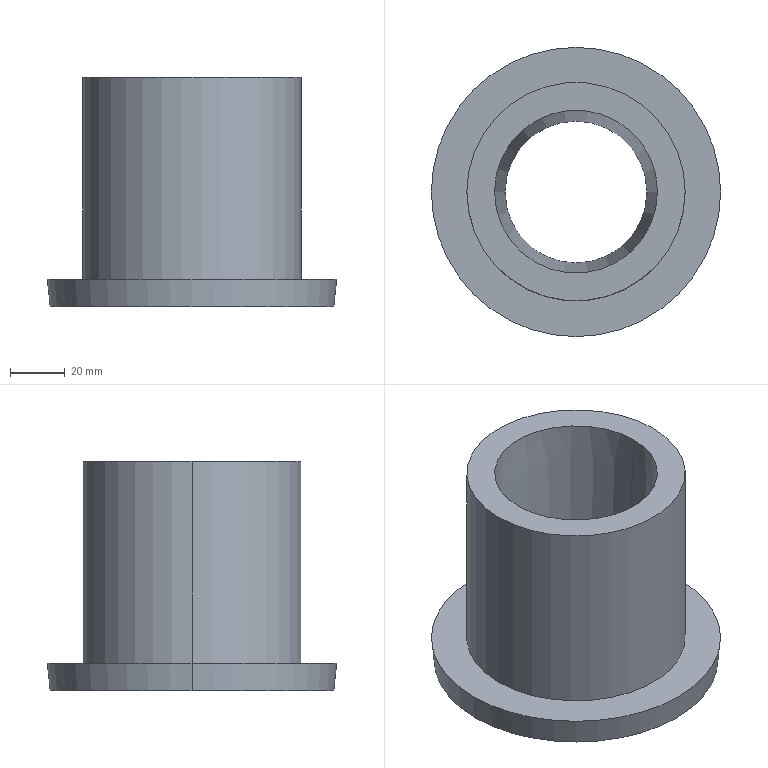Part | SolidWorks | features Revolution 1 | 1 solid | 9 faces | box 106 x 106 x 84 mm | volume 252355 mm3 | cone 4 | plane 3 | cylinder 2 | commonest cylinder face diameters 80 x2
STEP:
#1=CARTESIAN_POINT('',(-40.,318.5,-90.5));
#2=VERTEX_POINT('',#1);
#3=CARTESIAN_POINT('',(40.,318.5,-90.5));
#4=VERTEX_POINT('',#3);
#5=CARTESIAN_POINT('',(0.,318.5,-90.5));
#6=DIRECTION('',(0.,0.,-1.));
#7=DIRECTION('',(-1.,0.,0.));
#8=AXIS2_PLACEMENT_3D('',#5,#6,#7);
#9=CIRCLE('',#8,40.);
#10=EDGE_CURVE('',#2,#4,#9,.T.);
#11=ORIENTED_EDGE('',*,*,#10,.T.);
#12=CARTESIAN_POINT('',(40.,318.5,-164.5));
#13=VERTEX_POINT('',#12);
#14=CARTESIAN_POINT('',(40.,318.5,-174.5));
#15=DIRECTION('',(0.,0.,-1.));
#16=VECTOR('',#15,1000.);
#17=LINE('',#14,#16);
#18=EDGE_CURVE('',#4,#13,#17,.T.);
#19=ORIENTED_EDGE('',*,*,#18,.T.);
#20=CARTESIAN_POINT('',(-40.,318.5,-164.5));
#21=VERTEX_POINT('',#20);
#22=CARTESIAN_POINT('',(0.,318.5,-164.5));
#23=DIRECTION('',(0.,0.,-1.));
#24=DIRECTION('',(-1.,0.,0.));
#25=AXIS2_PLACEMENT_3D('',#22,#23,#24);
#26=CIRCLE('',#25,40.);
#27=EDGE_CURVE('',#21,#13,#26,.T.);
#28=ORIENTED_EDGE('',*,*,#27,.F.);
#29=CARTESIAN_POINT('',(-40.,318.5,-174.5));
#30=DIRECTION('',(0.,0.,-1.));
#31=VECTOR('',#30,1000.);
#32=LINE('',#29,#31);
#33=EDGE_CURVE('',#2,#21,#32,.T.);
#34=ORIENTED_EDGE('',*,*,#33,.F.);
#35=EDGE_LOOP('',(#11,#19,#28,#34));
#36=FACE_OUTER_BOUND('',#35,.T.);
#37=CARTESIAN_POINT('',(0.,318.5,-174.5));
#38=DIRECTION('',(0.,0.,-1.));
#39=DIRECTION('',(-1.,0.,0.));
#40=AXIS2_PLACEMENT_3D('',#37,#38,#39);
#41=CYLINDRICAL_SURFACE('',#40,40.);
#42=ADVANCED_FACE('',(#36),#41,.T.);
#43=CARTESIAN_POINT('',(-52.,318.5,-174.5));
#44=VERTEX_POINT('',#43);
#45=CARTESIAN_POINT('',(52.,318.5,-174.5));
#46=VERTEX_POINT('',#45);
#47=CARTESIAN_POINT('',(0.,318.5,-174.5));
#48=DIRECTION('',(0.,0.,-1.));
#49=DIRECTION('',(-1.,0.,0.));
#50=AXIS2_PLACEMENT_3D('',#47,#48,#49);
#51=CIRCLE('',#50,52.);
#52=EDGE_CURVE('',#44,#46,#51,.T.);
#53=ORIENTED_EDGE('',*,*,#52,.F.);
#54=CARTESIAN_POINT('',(-53.,318.5,-164.5));
#55=VERTEX_POINT('',#54);
#56=CARTESIAN_POINT('',(-53.,318.5,-164.5));
#57=DIRECTION('',(-0.0995,0.,0.995));
#58=VECTOR('',#57,1000.);
#59=LINE('',#56,#58);
#60=EDGE_CURVE('',#44,#55,#59,.T.);
#61=ORIENTED_EDGE('',*,*,#60,.T.);
#62=CARTESIAN_POINT('',(53.,318.5,-164.5));
#63=VERTEX_POINT('',#62);
#64=CARTESIAN_POINT('',(0.,318.5,-164.5));
#65=DIRECTION('',(0.,0.,-1.));
#66=DIRECTION('',(-1.,0.,0.));
#67=AXIS2_PLACEMENT_3D('',#64,#65,#66);
#68=CIRCLE('',#67,53.);
#69=EDGE_CURVE('',#55,#63,#68,.T.);
#70=ORIENTED_EDGE('',*,*,#69,.T.);
#71=CARTESIAN_POINT('',(53.,318.5,-164.5));
#72=DIRECTION('',(0.0995,0.,0.995));
#73=VECTOR('',#72,1000.);
#74=LINE('',#71,#73);
#75=EDGE_CURVE('',#46,#63,#74,.T.);
#76=ORIENTED_EDGE('',*,*,#75,.F.);
#77=EDGE_LOOP('',(#53,#61,#70,#76));
#78=FACE_OUTER_BOUND('',#77,.T.);
#79=CARTESIAN_POINT('',(0.,318.5,-164.5));
#80=DIRECTION('',(0.,0.,1.));
#81=DIRECTION('',(1.,0.,0.));
#82=AXIS2_PLACEMENT_3D('',#79,#80,#81);
#83=CONICAL_SURFACE('',#82,53.,0.09967);
#84=ADVANCED_FACE('',(#78),#83,.T.);
#85=CARTESIAN_POINT('',(26.,318.5,-174.5));
#86=VERTEX_POINT('',#85);
#87=CARTESIAN_POINT('',(-26.,318.5,-174.5));
#88=VERTEX_POINT('',#87);
#89=CARTESIAN_POINT('',(0.,318.5,-174.5));
#90=DIRECTION('',(0.,0.,-1.));
#91=DIRECTION('',(-1.,0.,0.));
#92=AXIS2_PLACEMENT_3D('',#89,#90,#91);
#93=CIRCLE('',#92,26.);
#94=EDGE_CURVE('',#86,#88,#93,.T.);
#95=ORIENTED_EDGE('',*,*,#94,.T.);
#96=CARTESIAN_POINT('',(-29.862,318.5,-90.5));
#97=VERTEX_POINT('',#96);
#98=CARTESIAN_POINT('',(-26.,318.5,-174.5));
#99=DIRECTION('',(-0.04593,0.,0.9989));
#100=VECTOR('',#99,1000.);
#101=LINE('',#98,#100);
#102=EDGE_CURVE('',#88,#97,#101,.T.);
#103=ORIENTED_EDGE('',*,*,#102,.T.);
#104=CARTESIAN_POINT('',(29.862,318.5,-90.5));
#105=VERTEX_POINT('',#104);
#106=CARTESIAN_POINT('',(0.,318.5,-90.5));
#107=DIRECTION('',(0.,0.,-1.));
#108=DIRECTION('',(-1.,0.,0.));
#109=AXIS2_PLACEMENT_3D('',#106,#107,#108);
#110=CIRCLE('',#109,29.862);
#111=EDGE_CURVE('',#105,#97,#110,.T.);
#112=ORIENTED_EDGE('',*,*,#111,.F.);
#113=CARTESIAN_POINT('',(26.,318.5,-174.5));
#114=DIRECTION('',(0.04593,0.,0.9989));
#115=VECTOR('',#114,1000.);
#116=LINE('',#113,#115);
#117=EDGE_CURVE('',#86,#105,#116,.T.);
#118=ORIENTED_EDGE('',*,*,#117,.F.);
#119=EDGE_LOOP('',(#95,#103,#112,#118));
#120=FACE_OUTER_BOUND('',#119,.T.);
#121=CARTESIAN_POINT('',(0.,318.5,-174.5));
#122=DIRECTION('',(0.,0.,1.));
#123=DIRECTION('',(1.,0.,0.));
#124=AXIS2_PLACEMENT_3D('',#121,#122,#123);
#125=CONICAL_SURFACE('',#124,26.,0.04594);
#126=ADVANCED_FACE('',(#120),#125,.F.);
#127=ORIENTED_EDGE('',*,*,#102,.F.);
#128=CARTESIAN_POINT('',(0.,318.5,-174.5));
#129=DIRECTION('',(0.,0.,-1.));
#130=DIRECTION('',(-1.,0.,0.));
#131=AXIS2_PLACEMENT_3D('',#128,#129,#130);
#132=CIRCLE('',#131,26.);
#133=EDGE_CURVE('',#88,#86,#132,.T.);
#134=ORIENTED_EDGE('',*,*,#133,.T.);
#135=ORIENTED_EDGE('',*,*,#117,.T.);
#136=CARTESIAN_POINT('',(0.,318.5,-90.5));
#137=DIRECTION('',(0.,0.,-1.));
#138=DIRECTION('',(-1.,0.,0.));
#139=AXIS2_PLACEMENT_3D('',#136,#137,#138);
#140=CIRCLE('',#139,29.862);
#141=EDGE_CURVE('',#97,#105,#140,.T.);
#142=ORIENTED_EDGE('',*,*,#141,.F.);
#143=EDGE_LOOP('',(#127,#134,#135,#142));
#144=FACE_OUTER_BOUND('',#143,.T.);
#145=CARTESIAN_POINT('',(0.,318.5,-174.5));
#146=DIRECTION('',(0.,0.,1.));
#147=DIRECTION('',(1.,0.,0.));
#148=AXIS2_PLACEMENT_3D('',#145,#146,#147);
#149=CONICAL_SURFACE('',#148,26.,0.04594);
#150=ADVANCED_FACE('',(#144),#149,.F.);
#151=ORIENTED_EDGE('',*,*,#94,.F.);
#152=ORIENTED_EDGE('',*,*,#133,.F.);
#153=EDGE_LOOP('',(#151,#152));
#154=FACE_BOUND('',#153,.T.);
#155=CARTESIAN_POINT('',(0.,318.5,-174.5));
#156=DIRECTION('',(0.,0.,-1.));
#157=DIRECTION('',(-1.,0.,0.));
#158=AXIS2_PLACEMENT_3D('',#155,#156,#157);
#159=CIRCLE('',#158,52.);
#160=EDGE_CURVE('',#46,#44,#159,.T.);
#161=ORIENTED_EDGE('',*,*,#160,.T.);
#162=ORIENTED_EDGE('',*,*,#52,.T.);
#163=EDGE_LOOP('',(#161,#162));
#164=FACE_OUTER_BOUND('',#163,.T.);
#165=CARTESIAN_POINT('',(-26.,318.5,-174.5));
#166=DIRECTION('',(0.,0.,1.));
#167=DIRECTION('',(1.,0.,0.));
#168=AXIS2_PLACEMENT_3D('',#165,#166,#167);
#169=PLANE('',#168);
#170=ADVANCED_FACE('',(#154,#164),#169,.F.);
#171=ORIENTED_EDGE('',*,*,#60,.F.);
#172=ORIENTED_EDGE('',*,*,#160,.F.);
#173=ORIENTED_EDGE('',*,*,#75,.T.);
#174=CARTESIAN_POINT('',(0.,318.5,-164.5));
#175=DIRECTION('',(0.,0.,-1.));
#176=DIRECTION('',(-1.,0.,0.));
#177=AXIS2_PLACEMENT_3D('',#174,#175,#176);
#178=CIRCLE('',#177,53.);
#179=EDGE_CURVE('',#63,#55,#178,.T.);
#180=ORIENTED_EDGE('',*,*,#179,.T.);
#181=EDGE_LOOP('',(#171,#172,#173,#180));
#182=FACE_OUTER_BOUND('',#181,.T.);
#183=CARTESIAN_POINT('',(0.,318.5,-164.5));
#184=DIRECTION('',(0.,0.,1.));
#185=DIRECTION('',(1.,0.,0.));
#186=AXIS2_PLACEMENT_3D('',#183,#184,#185);
#187=CONICAL_SURFACE('',#186,53.,0.09967);
#188=ADVANCED_FACE('',(#182),#187,.T.);
#189=ORIENTED_EDGE('',*,*,#179,.F.);
#190=ORIENTED_EDGE('',*,*,#69,.F.);
#191=EDGE_LOOP('',(#189,#190));
#192=FACE_OUTER_BOUND('',#191,.T.);
#193=ORIENTED_EDGE('',*,*,#27,.T.);
#194=CARTESIAN_POINT('',(0.,318.5,-164.5));
#195=DIRECTION('',(0.,0.,-1.));
#196=DIRECTION('',(-1.,0.,0.));
#197=AXIS2_PLACEMENT_3D('',#194,#195,#196);
#198=CIRCLE('',#197,40.);
#199=EDGE_CURVE('',#13,#21,#198,.T.);
#200=ORIENTED_EDGE('',*,*,#199,.T.);
#201=EDGE_LOOP('',(#193,#200));
#202=FACE_BOUND('',#201,.T.);
#203=CARTESIAN_POINT('',(-53.,318.5,-164.5));
#204=DIRECTION('',(0.,0.,-1.));
#205=DIRECTION('',(-1.,0.,0.));
#206=AXIS2_PLACEMENT_3D('',#203,#204,#205);
#207=PLANE('',#206);
#208=ADVANCED_FACE('',(#192,#202),#207,.F.);
#209=ORIENTED_EDGE('',*,*,#18,.F.);
#210=CARTESIAN_POINT('',(0.,318.5,-90.5));
#211=DIRECTION('',(0.,0.,-1.));
#212=DIRECTION('',(-1.,0.,0.));
#213=AXIS2_PLACEMENT_3D('',#210,#211,#212);
#214=CIRCLE('',#213,40.);
#215=EDGE_CURVE('',#4,#2,#214,.T.);
#216=ORIENTED_EDGE('',*,*,#215,.T.);
#217=ORIENTED_EDGE('',*,*,#33,.T.);
#218=ORIENTED_EDGE('',*,*,#199,.F.);
#219=EDGE_LOOP('',(#209,#216,#217,#218));
#220=FACE_OUTER_BOUND('',#219,.T.);
#221=CARTESIAN_POINT('',(0.,318.5,-174.5));
#222=DIRECTION('',(0.,0.,-1.));
#223=DIRECTION('',(-1.,0.,0.));
#224=AXIS2_PLACEMENT_3D('',#221,#222,#223);
#225=CYLINDRICAL_SURFACE('',#224,40.);
#226=ADVANCED_FACE('',(#220),#225,.T.);
#227=ORIENTED_EDGE('',*,*,#10,.F.);
#228=ORIENTED_EDGE('',*,*,#215,.F.);
#229=EDGE_LOOP('',(#227,#228));
#230=FACE_OUTER_BOUND('',#229,.T.);
#231=ORIENTED_EDGE('',*,*,#111,.T.);
#232=ORIENTED_EDGE('',*,*,#141,.T.);
#233=EDGE_LOOP('',(#231,#232));
#234=FACE_BOUND('',#233,.T.);
#235=CARTESIAN_POINT('',(-40.,318.5,-90.5));
#236=DIRECTION('',(0.,0.,-1.));
#237=DIRECTION('',(-1.,0.,0.));
#238=AXIS2_PLACEMENT_3D('',#235,#236,#237);
#239=PLANE('',#238);
#240=ADVANCED_FACE('',(#230,#234),#239,.F.);
#241=CLOSED_SHELL('',(#42,#84,#126,#150,#170,#188,#208,#226,#240));
#242=MANIFOLD_SOLID_BREP('',#241);
#243=CARTESIAN_POINT('',(0.,0.,0.));
#244=DIRECTION('',(0.,0.,1.));
#245=DIRECTION('',(1.,0.,0.));
#246=AXIS2_PLACEMENT_3D('',#243,#244,#245);
#247=(LENGTH_UNIT()NAMED_UNIT(*)SI_UNIT(.MILLI.,.METRE.));
#248=UNCERTAINTY_MEASURE_WITH_UNIT(LENGTH_MEASURE(0.00001),#247,'','');
#249=(NAMED_UNIT(*)PLANE_ANGLE_UNIT()SI_UNIT($,.RADIAN.));
#250=(NAMED_UNIT(*)SI_UNIT($,.STERADIAN.)SOLID_ANGLE_UNIT());
#251=(GEOMETRIC_REPRESENTATION_CONTEXT(3)GLOBAL_UNCERTAINTY_ASSIGNED_CONTEXT((#248))GLOBAL_UNIT_ASSIGNED_CONTEXT((#247,#249,#250))REPRESENTATION_CONTEXT('',''));
#252=ADVANCED_BREP_SHAPE_REPRESENTATION('',(#242,#246),#251);